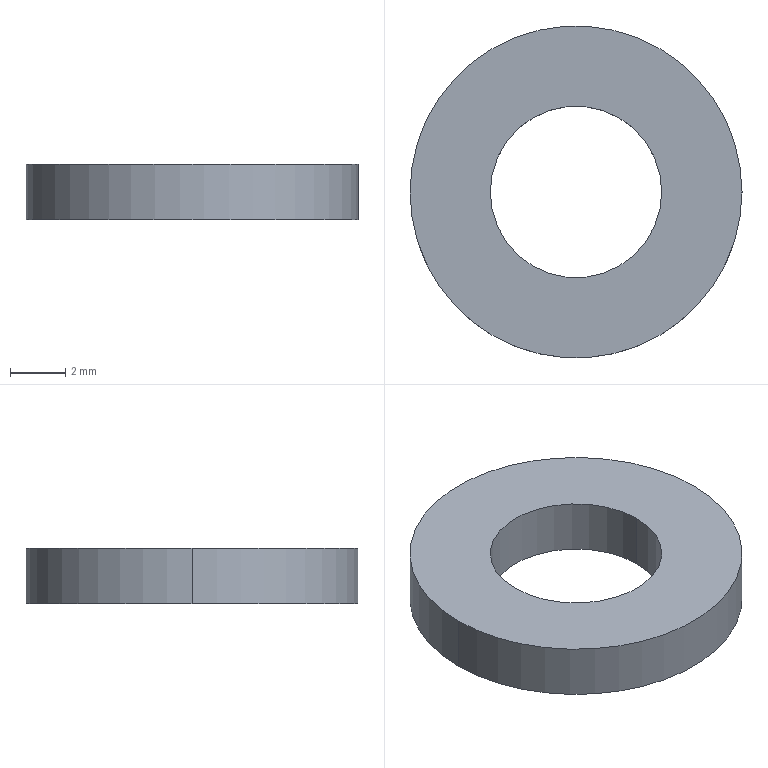Part | SolidWorks | features Extrusion 1 | 1 solid | 6 faces | box 12 x 12 x 2 mm | volume 165.813 mm3 | cylinder 4 | plane 2 | commonest cylinder face diameters 6.2 x2 12 x2
STEP:
#1=CARTESIAN_POINT('',(-3.1,0.,2.));
#2=VERTEX_POINT('',#1);
#3=CARTESIAN_POINT('',(3.1,0.,2.));
#4=VERTEX_POINT('',#3);
#5=CARTESIAN_POINT('',(0.,0.,2.));
#6=DIRECTION('',(0.,0.,1.));
#7=DIRECTION('',(1.,0.,0.));
#8=AXIS2_PLACEMENT_3D('',#5,#6,#7);
#9=CIRCLE('',#8,3.1);
#10=EDGE_CURVE('',#2,#4,#9,.T.);
#11=ORIENTED_EDGE('',*,*,#10,.T.);
#12=CARTESIAN_POINT('',(3.1,0.,0.));
#13=VERTEX_POINT('',#12);
#14=CARTESIAN_POINT('',(3.1,0.,2.));
#15=DIRECTION('',(0.,0.,-1.));
#16=VECTOR('',#15,1000.);
#17=LINE('',#14,#16);
#18=EDGE_CURVE('',#4,#13,#17,.T.);
#19=ORIENTED_EDGE('',*,*,#18,.T.);
#20=CARTESIAN_POINT('',(-3.1,0.,0.));
#21=VERTEX_POINT('',#20);
#22=CARTESIAN_POINT('',(0.,0.,0.));
#23=DIRECTION('',(0.,0.,1.));
#24=DIRECTION('',(1.,0.,0.));
#25=AXIS2_PLACEMENT_3D('',#22,#23,#24);
#26=CIRCLE('',#25,3.1);
#27=EDGE_CURVE('',#21,#13,#26,.T.);
#28=ORIENTED_EDGE('',*,*,#27,.F.);
#29=CARTESIAN_POINT('',(-3.1,0.,2.));
#30=DIRECTION('',(0.,0.,-1.));
#31=VECTOR('',#30,1000.);
#32=LINE('',#29,#31);
#33=EDGE_CURVE('',#2,#21,#32,.T.);
#34=ORIENTED_EDGE('',*,*,#33,.F.);
#35=EDGE_LOOP('',(#11,#19,#28,#34));
#36=FACE_OUTER_BOUND('',#35,.T.);
#37=CARTESIAN_POINT('',(0.,0.,2.));
#38=DIRECTION('',(0.,0.,-1.));
#39=DIRECTION('',(-1.,0.,0.));
#40=AXIS2_PLACEMENT_3D('',#37,#38,#39);
#41=CYLINDRICAL_SURFACE('',#40,3.1);
#42=ADVANCED_FACE('',(#36),#41,.F.);
#43=CARTESIAN_POINT('',(6.,0.,2.));
#44=VERTEX_POINT('',#43);
#45=CARTESIAN_POINT('',(-6.,0.,2.));
#46=VERTEX_POINT('',#45);
#47=CARTESIAN_POINT('',(0.,0.,2.));
#48=DIRECTION('',(0.,0.,1.));
#49=DIRECTION('',(1.,0.,0.));
#50=AXIS2_PLACEMENT_3D('',#47,#48,#49);
#51=CIRCLE('',#50,6.);
#52=EDGE_CURVE('',#44,#46,#51,.T.);
#53=ORIENTED_EDGE('',*,*,#52,.F.);
#54=CARTESIAN_POINT('',(6.,0.,0.));
#55=VERTEX_POINT('',#54);
#56=CARTESIAN_POINT('',(6.,0.,2.));
#57=DIRECTION('',(0.,0.,-1.));
#58=VECTOR('',#57,1000.);
#59=LINE('',#56,#58);
#60=EDGE_CURVE('',#44,#55,#59,.T.);
#61=ORIENTED_EDGE('',*,*,#60,.T.);
#62=CARTESIAN_POINT('',(-6.,0.,0.));
#63=VERTEX_POINT('',#62);
#64=CARTESIAN_POINT('',(0.,0.,0.));
#65=DIRECTION('',(0.,0.,1.));
#66=DIRECTION('',(1.,0.,0.));
#67=AXIS2_PLACEMENT_3D('',#64,#65,#66);
#68=CIRCLE('',#67,6.);
#69=EDGE_CURVE('',#55,#63,#68,.T.);
#70=ORIENTED_EDGE('',*,*,#69,.T.);
#71=CARTESIAN_POINT('',(-6.,0.,2.));
#72=DIRECTION('',(0.,0.,-1.));
#73=VECTOR('',#72,1000.);
#74=LINE('',#71,#73);
#75=EDGE_CURVE('',#46,#63,#74,.T.);
#76=ORIENTED_EDGE('',*,*,#75,.F.);
#77=EDGE_LOOP('',(#53,#61,#70,#76));
#78=FACE_OUTER_BOUND('',#77,.T.);
#79=CARTESIAN_POINT('',(0.,0.,2.));
#80=DIRECTION('',(0.,0.,-1.));
#81=DIRECTION('',(-1.,0.,0.));
#82=AXIS2_PLACEMENT_3D('',#79,#80,#81);
#83=CYLINDRICAL_SURFACE('',#82,6.);
#84=ADVANCED_FACE('',(#78),#83,.T.);
#85=CARTESIAN_POINT('',(0.,0.,2.));
#86=DIRECTION('',(0.,0.,1.));
#87=DIRECTION('',(1.,0.,0.));
#88=AXIS2_PLACEMENT_3D('',#85,#86,#87);
#89=CIRCLE('',#88,6.);
#90=EDGE_CURVE('',#46,#44,#89,.T.);
#91=ORIENTED_EDGE('',*,*,#90,.T.);
#92=ORIENTED_EDGE('',*,*,#52,.T.);
#93=EDGE_LOOP('',(#91,#92));
#94=FACE_OUTER_BOUND('',#93,.T.);
#95=ORIENTED_EDGE('',*,*,#10,.F.);
#96=CARTESIAN_POINT('',(0.,0.,2.));
#97=DIRECTION('',(0.,0.,1.));
#98=DIRECTION('',(1.,0.,0.));
#99=AXIS2_PLACEMENT_3D('',#96,#97,#98);
#100=CIRCLE('',#99,3.1);
#101=EDGE_CURVE('',#4,#2,#100,.T.);
#102=ORIENTED_EDGE('',*,*,#101,.F.);
#103=EDGE_LOOP('',(#95,#102));
#104=FACE_BOUND('',#103,.T.);
#105=CARTESIAN_POINT('',(0.,0.,2.));
#106=DIRECTION('',(0.,0.,1.));
#107=DIRECTION('',(1.,0.,0.));
#108=AXIS2_PLACEMENT_3D('',#105,#106,#107);
#109=PLANE('',#108);
#110=ADVANCED_FACE('',(#94,#104),#109,.T.);
#111=CARTESIAN_POINT('',(0.,0.,0.));
#112=DIRECTION('',(0.,0.,1.));
#113=DIRECTION('',(1.,0.,0.));
#114=AXIS2_PLACEMENT_3D('',#111,#112,#113);
#115=CIRCLE('',#114,6.);
#116=EDGE_CURVE('',#63,#55,#115,.T.);
#117=ORIENTED_EDGE('',*,*,#116,.F.);
#118=ORIENTED_EDGE('',*,*,#69,.F.);
#119=EDGE_LOOP('',(#117,#118));
#120=FACE_OUTER_BOUND('',#119,.T.);
#121=ORIENTED_EDGE('',*,*,#27,.T.);
#122=CARTESIAN_POINT('',(0.,0.,0.));
#123=DIRECTION('',(0.,0.,1.));
#124=DIRECTION('',(1.,0.,0.));
#125=AXIS2_PLACEMENT_3D('',#122,#123,#124);
#126=CIRCLE('',#125,3.1);
#127=EDGE_CURVE('',#13,#21,#126,.T.);
#128=ORIENTED_EDGE('',*,*,#127,.T.);
#129=EDGE_LOOP('',(#121,#128));
#130=FACE_BOUND('',#129,.T.);
#131=CARTESIAN_POINT('',(0.,0.,0.));
#132=DIRECTION('',(0.,0.,1.));
#133=DIRECTION('',(1.,0.,0.));
#134=AXIS2_PLACEMENT_3D('',#131,#132,#133);
#135=PLANE('',#134);
#136=ADVANCED_FACE('',(#120,#130),#135,.F.);
#137=ORIENTED_EDGE('',*,*,#60,.F.);
#138=ORIENTED_EDGE('',*,*,#90,.F.);
#139=ORIENTED_EDGE('',*,*,#75,.T.);
#140=ORIENTED_EDGE('',*,*,#116,.T.);
#141=EDGE_LOOP('',(#137,#138,#139,#140));
#142=FACE_OUTER_BOUND('',#141,.T.);
#143=CARTESIAN_POINT('',(0.,0.,2.));
#144=DIRECTION('',(0.,0.,-1.));
#145=DIRECTION('',(-1.,0.,0.));
#146=AXIS2_PLACEMENT_3D('',#143,#144,#145);
#147=CYLINDRICAL_SURFACE('',#146,6.);
#148=ADVANCED_FACE('',(#142),#147,.T.);
#149=ORIENTED_EDGE('',*,*,#18,.F.);
#150=ORIENTED_EDGE('',*,*,#101,.T.);
#151=ORIENTED_EDGE('',*,*,#33,.T.);
#152=ORIENTED_EDGE('',*,*,#127,.F.);
#153=EDGE_LOOP('',(#149,#150,#151,#152));
#154=FACE_OUTER_BOUND('',#153,.T.);
#155=CARTESIAN_POINT('',(0.,0.,2.));
#156=DIRECTION('',(0.,0.,-1.));
#157=DIRECTION('',(-1.,0.,0.));
#158=AXIS2_PLACEMENT_3D('',#155,#156,#157);
#159=CYLINDRICAL_SURFACE('',#158,3.1);
#160=ADVANCED_FACE('',(#154),#159,.F.);
#161=CLOSED_SHELL('',(#42,#84,#110,#136,#148,#160));
#162=MANIFOLD_SOLID_BREP('',#161);
#163=CARTESIAN_POINT('',(0.,0.,0.));
#164=DIRECTION('',(0.,0.,1.));
#165=DIRECTION('',(1.,0.,0.));
#166=AXIS2_PLACEMENT_3D('',#163,#164,#165);
#167=(LENGTH_UNIT()NAMED_UNIT(*)SI_UNIT(.MILLI.,.METRE.));
#168=UNCERTAINTY_MEASURE_WITH_UNIT(LENGTH_MEASURE(0.00001),#167,'','');
#169=(NAMED_UNIT(*)PLANE_ANGLE_UNIT()SI_UNIT($,.RADIAN.));
#170=(NAMED_UNIT(*)SI_UNIT($,.STERADIAN.)SOLID_ANGLE_UNIT());
#171=(GEOMETRIC_REPRESENTATION_CONTEXT(3)GLOBAL_UNCERTAINTY_ASSIGNED_CONTEXT((#168))GLOBAL_UNIT_ASSIGNED_CONTEXT((#167,#169,#170))REPRESENTATION_CONTEXT('',''));
#172=ADVANCED_BREP_SHAPE_REPRESENTATION('',(#162,#166),#171);